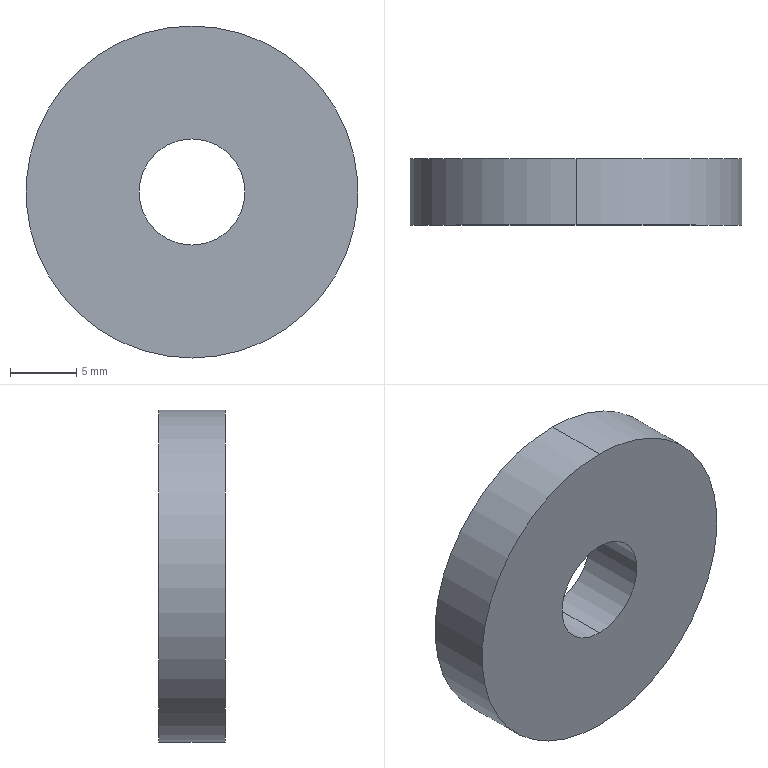Part | STEP file | PN_0001_default | 1 solid | 6 faces | box 25 x 5 x 25 mm | volume 2203 mm3 | cylinder 4 | plane 2 | commonest cylinder face diameters 8 x2 25 x2
STEP:
#1=CARTESIAN_POINT('',(0.,0.,0.));
#2=DIRECTION('',(0.,0.,1.));
#3=DIRECTION('',(1.,0.,0.));
#4=AXIS2_PLACEMENT_3D('',#1,#2,#3);
#5=CARTESIAN_POINT('',(0.,5.,-4.));
#6=VERTEX_POINT('',#5);
#7=CARTESIAN_POINT('',(0.,0.,-4.));
#8=VERTEX_POINT('',#7);
#9=CARTESIAN_POINT('',(0.,5.,-4.));
#10=DIRECTION('',(0.,-1.,0.));
#11=VECTOR('',#10,1.);
#12=LINE('',#9,#11);
#13=CARTESIAN_POINT('',(0.,5.,0.));
#14=DIRECTION('',(0.,-1.,0.));
#15=DIRECTION('',(0.,0.,-1.));
#16=AXIS2_PLACEMENT_3D('',#13,#14,#15);
#17=CYLINDRICAL_SURFACE('',#16,4.);
#18=CARTESIAN_POINT('',(6.283,0.));
#19=DIRECTION('',(0.,1.));
#20=VECTOR('',#19,1.);
#21=LINE('',#18,#20);
#22=(GEOMETRIC_REPRESENTATION_CONTEXT(2)PARAMETRIC_REPRESENTATION_CONTEXT()REPRESENTATION_CONTEXT('',''));
#23=DEFINITIONAL_REPRESENTATION('',(#21),#22);
#24=PCURVE('',#17,#23);
#25=CARTESIAN_POINT('',(0.,5.,0.));
#26=DIRECTION('',(0.,-1.,0.));
#27=DIRECTION('',(0.,0.,-1.));
#28=AXIS2_PLACEMENT_3D('',#25,#26,#27);
#29=CYLINDRICAL_SURFACE('',#28,4.);
#30=CARTESIAN_POINT('',(0.,0.));
#31=DIRECTION('',(0.,1.));
#32=VECTOR('',#31,1.);
#33=LINE('',#30,#32);
#34=(GEOMETRIC_REPRESENTATION_CONTEXT(2)PARAMETRIC_REPRESENTATION_CONTEXT()REPRESENTATION_CONTEXT('',''));
#35=DEFINITIONAL_REPRESENTATION('',(#33),#34);
#36=PCURVE('',#29,#35);
#37=SURFACE_CURVE('',#12,(#24,#36),.PCURVE_S1.);
#38=EDGE_CURVE('',#6,#8,#37,.T.);
#39=ORIENTED_EDGE('',*,*,#38,.T.);
#40=CARTESIAN_POINT('',(0.,0.,4.));
#41=VERTEX_POINT('',#40);
#42=CARTESIAN_POINT('',(0.,0.,0.));
#43=DIRECTION('',(0.,1.,0.));
#44=DIRECTION('',(0.,0.,1.));
#45=AXIS2_PLACEMENT_3D('',#42,#43,#44);
#46=CIRCLE('',#45,4.);
#47=CARTESIAN_POINT('',(9.425,5.));
#48=DIRECTION('',(-1.,0.));
#49=VECTOR('',#48,1.);
#50=LINE('',#47,#49);
#51=(GEOMETRIC_REPRESENTATION_CONTEXT(2)PARAMETRIC_REPRESENTATION_CONTEXT()REPRESENTATION_CONTEXT('',''));
#52=DEFINITIONAL_REPRESENTATION('',(#50),#51);
#53=PCURVE('',#17,#52);
#54=CARTESIAN_POINT('',(0.,0.,0.));
#55=DIRECTION('',(0.,1.,0.));
#56=DIRECTION('',(0.,0.,1.));
#57=AXIS2_PLACEMENT_3D('',#54,#55,#56);
#58=PLANE('',#57);
#59=CARTESIAN_POINT('',(0.,0.));
#60=DIRECTION('',(1.,0.));
#61=AXIS2_PLACEMENT_2D('',#59,#60);
#62=CIRCLE('',#61,4.);
#63=(GEOMETRIC_REPRESENTATION_CONTEXT(2)PARAMETRIC_REPRESENTATION_CONTEXT()REPRESENTATION_CONTEXT('',''));
#64=DEFINITIONAL_REPRESENTATION('',(#62),#63);
#65=PCURVE('',#58,#64);
#66=SURFACE_CURVE('',#46,(#53,#65),.PCURVE_S1.);
#67=EDGE_CURVE('',#8,#41,#66,.T.);
#68=ORIENTED_EDGE('',*,*,#67,.T.);
#69=CARTESIAN_POINT('',(0.,5.,4.));
#70=VERTEX_POINT('',#69);
#71=CARTESIAN_POINT('',(0.,5.,4.));
#72=DIRECTION('',(0.,-1.,0.));
#73=VECTOR('',#72,1.);
#74=LINE('',#71,#73);
#75=CARTESIAN_POINT('',(3.142,0.));
#76=DIRECTION('',(0.,1.));
#77=VECTOR('',#76,1.);
#78=LINE('',#75,#77);
#79=(GEOMETRIC_REPRESENTATION_CONTEXT(2)PARAMETRIC_REPRESENTATION_CONTEXT()REPRESENTATION_CONTEXT('',''));
#80=DEFINITIONAL_REPRESENTATION('',(#78),#79);
#81=PCURVE('',#17,#80);
#82=CARTESIAN_POINT('',(3.142,0.));
#83=DIRECTION('',(0.,1.));
#84=VECTOR('',#83,1.);
#85=LINE('',#82,#84);
#86=(GEOMETRIC_REPRESENTATION_CONTEXT(2)PARAMETRIC_REPRESENTATION_CONTEXT()REPRESENTATION_CONTEXT('',''));
#87=DEFINITIONAL_REPRESENTATION('',(#85),#86);
#88=PCURVE('',#29,#87);
#89=SURFACE_CURVE('',#74,(#81,#88),.PCURVE_S1.);
#90=EDGE_CURVE('',#70,#41,#89,.T.);
#91=ORIENTED_EDGE('',*,*,#90,.F.);
#92=CARTESIAN_POINT('',(0.,5.,0.));
#93=DIRECTION('',(0.,1.,0.));
#94=DIRECTION('',(0.,0.,1.));
#95=AXIS2_PLACEMENT_3D('',#92,#93,#94);
#96=CIRCLE('',#95,4.);
#97=CARTESIAN_POINT('',(9.425,0.));
#98=DIRECTION('',(-1.,0.));
#99=VECTOR('',#98,1.);
#100=LINE('',#97,#99);
#101=(GEOMETRIC_REPRESENTATION_CONTEXT(2)PARAMETRIC_REPRESENTATION_CONTEXT()REPRESENTATION_CONTEXT('',''));
#102=DEFINITIONAL_REPRESENTATION('',(#100),#101);
#103=PCURVE('',#17,#102);
#104=CARTESIAN_POINT('',(0.,5.,0.));
#105=DIRECTION('',(0.,1.,0.));
#106=DIRECTION('',(0.,0.,1.));
#107=AXIS2_PLACEMENT_3D('',#104,#105,#106);
#108=PLANE('',#107);
#109=CARTESIAN_POINT('',(0.,0.));
#110=DIRECTION('',(1.,0.));
#111=AXIS2_PLACEMENT_2D('',#109,#110);
#112=CIRCLE('',#111,4.);
#113=(GEOMETRIC_REPRESENTATION_CONTEXT(2)PARAMETRIC_REPRESENTATION_CONTEXT()REPRESENTATION_CONTEXT('',''));
#114=DEFINITIONAL_REPRESENTATION('',(#112),#113);
#115=PCURVE('',#108,#114);
#116=SURFACE_CURVE('',#96,(#103,#115),.PCURVE_S1.);
#117=EDGE_CURVE('',#6,#70,#116,.T.);
#118=ORIENTED_EDGE('',*,*,#117,.F.);
#119=EDGE_LOOP('',(#39,#68,#91,#118));
#120=FACE_BOUND('',#119,.F.);
#121=ADVANCED_FACE('',(#120),#17,.F.);
#122=CARTESIAN_POINT('',(0.,5.,12.5));
#123=VERTEX_POINT('',#122);
#124=CARTESIAN_POINT('',(0.,5.,-12.5));
#125=VERTEX_POINT('',#124);
#126=CARTESIAN_POINT('',(0.,5.,0.));
#127=DIRECTION('',(0.,1.,0.));
#128=DIRECTION('',(0.,0.,1.));
#129=AXIS2_PLACEMENT_3D('',#126,#127,#128);
#130=CIRCLE('',#129,12.5);
#131=CARTESIAN_POINT('',(0.,5.,0.));
#132=DIRECTION('',(0.,-1.,0.));
#133=DIRECTION('',(0.,0.,-1.));
#134=AXIS2_PLACEMENT_3D('',#131,#132,#133);
#135=CYLINDRICAL_SURFACE('',#134,12.5);
#136=CARTESIAN_POINT('',(3.142,0.));
#137=DIRECTION('',(-1.,0.));
#138=VECTOR('',#137,1.);
#139=LINE('',#136,#138);
#140=(GEOMETRIC_REPRESENTATION_CONTEXT(2)PARAMETRIC_REPRESENTATION_CONTEXT()REPRESENTATION_CONTEXT('',''));
#141=DEFINITIONAL_REPRESENTATION('',(#139),#140);
#142=PCURVE('',#135,#141);
#143=CARTESIAN_POINT('',(0.,0.));
#144=DIRECTION('',(1.,0.));
#145=AXIS2_PLACEMENT_2D('',#143,#144);
#146=CIRCLE('',#145,12.5);
#147=(GEOMETRIC_REPRESENTATION_CONTEXT(2)PARAMETRIC_REPRESENTATION_CONTEXT()REPRESENTATION_CONTEXT('',''));
#148=DEFINITIONAL_REPRESENTATION('',(#146),#147);
#149=PCURVE('',#108,#148);
#150=SURFACE_CURVE('',#130,(#142,#149),.PCURVE_S1.);
#151=EDGE_CURVE('',#123,#125,#150,.T.);
#152=ORIENTED_EDGE('',*,*,#151,.F.);
#153=CARTESIAN_POINT('',(0.,0.,12.5));
#154=VERTEX_POINT('',#153);
#155=CARTESIAN_POINT('',(0.,5.,12.5));
#156=DIRECTION('',(0.,-1.,0.));
#157=VECTOR('',#156,1.);
#158=LINE('',#155,#157);
#159=CARTESIAN_POINT('',(3.142,0.));
#160=DIRECTION('',(0.,1.));
#161=VECTOR('',#160,1.);
#162=LINE('',#159,#161);
#163=(GEOMETRIC_REPRESENTATION_CONTEXT(2)PARAMETRIC_REPRESENTATION_CONTEXT()REPRESENTATION_CONTEXT('',''));
#164=DEFINITIONAL_REPRESENTATION('',(#162),#163);
#165=PCURVE('',#135,#164);
#166=CARTESIAN_POINT('',(0.,5.,0.));
#167=DIRECTION('',(0.,-1.,0.));
#168=DIRECTION('',(0.,0.,-1.));
#169=AXIS2_PLACEMENT_3D('',#166,#167,#168);
#170=CYLINDRICAL_SURFACE('',#169,12.5);
#171=CARTESIAN_POINT('',(3.142,0.));
#172=DIRECTION('',(0.,1.));
#173=VECTOR('',#172,1.);
#174=LINE('',#171,#173);
#175=(GEOMETRIC_REPRESENTATION_CONTEXT(2)PARAMETRIC_REPRESENTATION_CONTEXT()REPRESENTATION_CONTEXT('',''));
#176=DEFINITIONAL_REPRESENTATION('',(#174),#175);
#177=PCURVE('',#170,#176);
#178=SURFACE_CURVE('',#158,(#165,#177),.PCURVE_S1.);
#179=EDGE_CURVE('',#123,#154,#178,.T.);
#180=ORIENTED_EDGE('',*,*,#179,.T.);
#181=CARTESIAN_POINT('',(0.,0.,-12.5));
#182=VERTEX_POINT('',#181);
#183=CARTESIAN_POINT('',(0.,0.,0.));
#184=DIRECTION('',(0.,1.,0.));
#185=DIRECTION('',(0.,0.,1.));
#186=AXIS2_PLACEMENT_3D('',#183,#184,#185);
#187=CIRCLE('',#186,12.5);
#188=CARTESIAN_POINT('',(3.142,5.));
#189=DIRECTION('',(-1.,0.));
#190=VECTOR('',#189,1.);
#191=LINE('',#188,#190);
#192=(GEOMETRIC_REPRESENTATION_CONTEXT(2)PARAMETRIC_REPRESENTATION_CONTEXT()REPRESENTATION_CONTEXT('',''));
#193=DEFINITIONAL_REPRESENTATION('',(#191),#192);
#194=PCURVE('',#135,#193);
#195=CARTESIAN_POINT('',(0.,0.));
#196=DIRECTION('',(1.,0.));
#197=AXIS2_PLACEMENT_2D('',#195,#196);
#198=CIRCLE('',#197,12.5);
#199=(GEOMETRIC_REPRESENTATION_CONTEXT(2)PARAMETRIC_REPRESENTATION_CONTEXT()REPRESENTATION_CONTEXT('',''));
#200=DEFINITIONAL_REPRESENTATION('',(#198),#199);
#201=PCURVE('',#58,#200);
#202=SURFACE_CURVE('',#187,(#194,#201),.PCURVE_S1.);
#203=EDGE_CURVE('',#154,#182,#202,.T.);
#204=ORIENTED_EDGE('',*,*,#203,.T.);
#205=CARTESIAN_POINT('',(0.,5.,-12.5));
#206=DIRECTION('',(0.,-1.,0.));
#207=VECTOR('',#206,1.);
#208=LINE('',#205,#207);
#209=CARTESIAN_POINT('',(0.,0.));
#210=DIRECTION('',(0.,1.));
#211=VECTOR('',#210,1.);
#212=LINE('',#209,#211);
#213=(GEOMETRIC_REPRESENTATION_CONTEXT(2)PARAMETRIC_REPRESENTATION_CONTEXT()REPRESENTATION_CONTEXT('',''));
#214=DEFINITIONAL_REPRESENTATION('',(#212),#213);
#215=PCURVE('',#135,#214);
#216=CARTESIAN_POINT('',(6.283,0.));
#217=DIRECTION('',(0.,1.));
#218=VECTOR('',#217,1.);
#219=LINE('',#216,#218);
#220=(GEOMETRIC_REPRESENTATION_CONTEXT(2)PARAMETRIC_REPRESENTATION_CONTEXT()REPRESENTATION_CONTEXT('',''));
#221=DEFINITIONAL_REPRESENTATION('',(#219),#220);
#222=PCURVE('',#170,#221);
#223=SURFACE_CURVE('',#208,(#215,#222),.PCURVE_S1.);
#224=EDGE_CURVE('',#125,#182,#223,.T.);
#225=ORIENTED_EDGE('',*,*,#224,.F.);
#226=EDGE_LOOP('',(#152,#180,#204,#225));
#227=FACE_BOUND('',#226,.T.);
#228=ADVANCED_FACE('',(#227),#135,.T.);
#229=CARTESIAN_POINT('',(0.,5.,0.));
#230=DIRECTION('',(0.,1.,0.));
#231=DIRECTION('',(0.,0.,1.));
#232=AXIS2_PLACEMENT_3D('',#229,#230,#231);
#233=CIRCLE('',#232,12.5);
#234=CARTESIAN_POINT('',(0.,0.));
#235=DIRECTION('',(1.,0.));
#236=AXIS2_PLACEMENT_2D('',#234,#235);
#237=CIRCLE('',#236,12.5);
#238=(GEOMETRIC_REPRESENTATION_CONTEXT(2)PARAMETRIC_REPRESENTATION_CONTEXT()REPRESENTATION_CONTEXT('',''));
#239=DEFINITIONAL_REPRESENTATION('',(#237),#238);
#240=PCURVE('',#108,#239);
#241=CARTESIAN_POINT('',(9.425,0.));
#242=DIRECTION('',(-1.,0.));
#243=VECTOR('',#242,1.);
#244=LINE('',#241,#243);
#245=(GEOMETRIC_REPRESENTATION_CONTEXT(2)PARAMETRIC_REPRESENTATION_CONTEXT()REPRESENTATION_CONTEXT('',''));
#246=DEFINITIONAL_REPRESENTATION('',(#244),#245);
#247=PCURVE('',#170,#246);
#248=SURFACE_CURVE('',#233,(#240,#247),.PCURVE_S1.);
#249=EDGE_CURVE('',#125,#123,#248,.T.);
#250=ORIENTED_EDGE('',*,*,#249,.T.);
#251=ORIENTED_EDGE('',*,*,#151,.T.);
#252=EDGE_LOOP('',(#250,#251));
#253=FACE_BOUND('',#252,.T.);
#254=ORIENTED_EDGE('',*,*,#117,.F.);
#255=CARTESIAN_POINT('',(0.,5.,0.));
#256=DIRECTION('',(0.,1.,0.));
#257=DIRECTION('',(0.,0.,1.));
#258=AXIS2_PLACEMENT_3D('',#255,#256,#257);
#259=CIRCLE('',#258,4.);
#260=CARTESIAN_POINT('',(0.,0.));
#261=DIRECTION('',(1.,0.));
#262=AXIS2_PLACEMENT_2D('',#260,#261);
#263=CIRCLE('',#262,4.);
#264=(GEOMETRIC_REPRESENTATION_CONTEXT(2)PARAMETRIC_REPRESENTATION_CONTEXT()REPRESENTATION_CONTEXT('',''));
#265=DEFINITIONAL_REPRESENTATION('',(#263),#264);
#266=PCURVE('',#108,#265);
#267=CARTESIAN_POINT('',(3.142,0.));
#268=DIRECTION('',(-1.,0.));
#269=VECTOR('',#268,1.);
#270=LINE('',#267,#269);
#271=(GEOMETRIC_REPRESENTATION_CONTEXT(2)PARAMETRIC_REPRESENTATION_CONTEXT()REPRESENTATION_CONTEXT('',''));
#272=DEFINITIONAL_REPRESENTATION('',(#270),#271);
#273=PCURVE('',#29,#272);
#274=SURFACE_CURVE('',#259,(#266,#273),.PCURVE_S1.);
#275=EDGE_CURVE('',#70,#6,#274,.T.);
#276=ORIENTED_EDGE('',*,*,#275,.F.);
#277=EDGE_LOOP('',(#254,#276));
#278=FACE_BOUND('',#277,.T.);
#279=ADVANCED_FACE('',(#253,#278),#108,.T.);
#280=CARTESIAN_POINT('',(0.,0.,0.));
#281=DIRECTION('',(0.,1.,0.));
#282=DIRECTION('',(0.,0.,1.));
#283=AXIS2_PLACEMENT_3D('',#280,#281,#282);
#284=CIRCLE('',#283,12.5);
#285=CARTESIAN_POINT('',(0.,0.));
#286=DIRECTION('',(1.,0.));
#287=AXIS2_PLACEMENT_2D('',#285,#286);
#288=CIRCLE('',#287,12.5);
#289=(GEOMETRIC_REPRESENTATION_CONTEXT(2)PARAMETRIC_REPRESENTATION_CONTEXT()REPRESENTATION_CONTEXT('',''));
#290=DEFINITIONAL_REPRESENTATION('',(#288),#289);
#291=PCURVE('',#58,#290);
#292=CARTESIAN_POINT('',(9.425,5.));
#293=DIRECTION('',(-1.,0.));
#294=VECTOR('',#293,1.);
#295=LINE('',#292,#294);
#296=(GEOMETRIC_REPRESENTATION_CONTEXT(2)PARAMETRIC_REPRESENTATION_CONTEXT()REPRESENTATION_CONTEXT('',''));
#297=DEFINITIONAL_REPRESENTATION('',(#295),#296);
#298=PCURVE('',#170,#297);
#299=SURFACE_CURVE('',#284,(#291,#298),.PCURVE_S1.);
#300=EDGE_CURVE('',#182,#154,#299,.T.);
#301=ORIENTED_EDGE('',*,*,#300,.F.);
#302=ORIENTED_EDGE('',*,*,#203,.F.);
#303=EDGE_LOOP('',(#301,#302));
#304=FACE_BOUND('',#303,.T.);
#305=ORIENTED_EDGE('',*,*,#67,.T.);
#306=CARTESIAN_POINT('',(0.,0.,0.));
#307=DIRECTION('',(0.,1.,0.));
#308=DIRECTION('',(0.,0.,1.));
#309=AXIS2_PLACEMENT_3D('',#306,#307,#308);
#310=CIRCLE('',#309,4.);
#311=CARTESIAN_POINT('',(0.,0.));
#312=DIRECTION('',(1.,0.));
#313=AXIS2_PLACEMENT_2D('',#311,#312);
#314=CIRCLE('',#313,4.);
#315=(GEOMETRIC_REPRESENTATION_CONTEXT(2)PARAMETRIC_REPRESENTATION_CONTEXT()REPRESENTATION_CONTEXT('',''));
#316=DEFINITIONAL_REPRESENTATION('',(#314),#315);
#317=PCURVE('',#58,#316);
#318=CARTESIAN_POINT('',(3.142,5.));
#319=DIRECTION('',(-1.,0.));
#320=VECTOR('',#319,1.);
#321=LINE('',#318,#320);
#322=(GEOMETRIC_REPRESENTATION_CONTEXT(2)PARAMETRIC_REPRESENTATION_CONTEXT()REPRESENTATION_CONTEXT('',''));
#323=DEFINITIONAL_REPRESENTATION('',(#321),#322);
#324=PCURVE('',#29,#323);
#325=SURFACE_CURVE('',#310,(#317,#324),.PCURVE_S1.);
#326=EDGE_CURVE('',#41,#8,#325,.T.);
#327=ORIENTED_EDGE('',*,*,#326,.T.);
#328=EDGE_LOOP('',(#305,#327));
#329=FACE_BOUND('',#328,.T.);
#330=ADVANCED_FACE('',(#304,#329),#58,.F.);
#331=ORIENTED_EDGE('',*,*,#179,.F.);
#332=ORIENTED_EDGE('',*,*,#249,.F.);
#333=ORIENTED_EDGE('',*,*,#224,.T.);
#334=ORIENTED_EDGE('',*,*,#300,.T.);
#335=EDGE_LOOP('',(#331,#332,#333,#334));
#336=FACE_BOUND('',#335,.T.);
#337=ADVANCED_FACE('',(#336),#170,.T.);
#338=ORIENTED_EDGE('',*,*,#326,.T.);
#339=ORIENTED_EDGE('',*,*,#38,.F.);
#340=ORIENTED_EDGE('',*,*,#275,.F.);
#341=ORIENTED_EDGE('',*,*,#90,.T.);
#342=EDGE_LOOP('',(#338,#339,#340,#341));
#343=FACE_BOUND('',#342,.F.);
#344=ADVANCED_FACE('',(#343),#29,.F.);
#345=CLOSED_SHELL('',(#121,#228,#279,#330,#337,#344));
#346=MANIFOLD_SOLID_BREP('',#345);
#347=(LENGTH_UNIT()NAMED_UNIT(*)SI_UNIT(.MILLI.,.METRE.));
#348=UNCERTAINTY_MEASURE_WITH_UNIT(LENGTH_MEASURE(0.0000001),#347,'','');
#349=(NAMED_UNIT(*)PLANE_ANGLE_UNIT()SI_UNIT($,.RADIAN.));
#350=(NAMED_UNIT(*)SI_UNIT($,.STERADIAN.)SOLID_ANGLE_UNIT());
#351=(GEOMETRIC_REPRESENTATION_CONTEXT(3)GLOBAL_UNCERTAINTY_ASSIGNED_CONTEXT((#348))GLOBAL_UNIT_ASSIGNED_CONTEXT((#347,#349,#350))REPRESENTATION_CONTEXT('',''));
#352=ADVANCED_BREP_SHAPE_REPRESENTATION('',(#4,#346),#351);